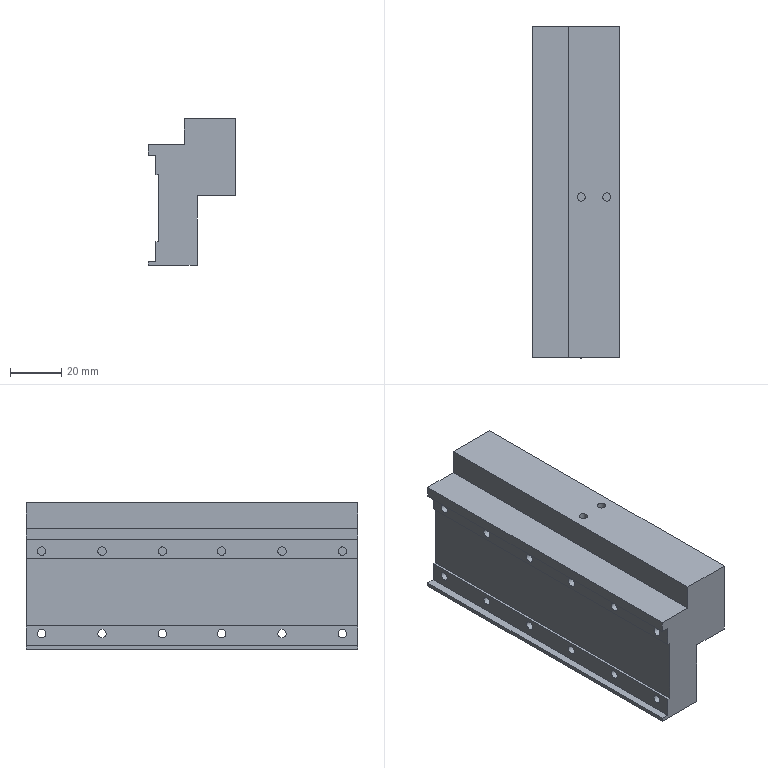Part | NX | 1 solid | 46 faces | box 34 x 129 x 57 mm | volume 157217 mm3 | plane 29 | cylinder 17 | commonest cylinder face diameters 3.3 x12 5 x3 3.2 x2
STEP:
#1=CARTESIAN_POINT('',(445.094,96.943,-207.9));
#2=VERTEX_POINT('',#1);
#3=CARTESIAN_POINT('',(446.694,96.943,-207.9));
#4=DIRECTION('',(0.,0.,-1.));
#5=DIRECTION('',(-1.,0.,0.));
#6=AXIS2_PLACEMENT_3D('',#3,#4,#5);
#7=CIRCLE('',#6,1.6);
#8=EDGE_CURVE('',#2,#2,#7,.T.);
#9=ORIENTED_EDGE('',*,*,#8,.F.);
#10=EDGE_LOOP('',(#9));
#11=FACE_BOUND('',#10,.T.);
#12=CARTESIAN_POINT('',(445.094,96.943,-215.9));
#13=VERTEX_POINT('',#12);
#14=CARTESIAN_POINT('',(446.694,96.943,-215.9));
#15=DIRECTION('',(0.,0.,-1.));
#16=DIRECTION('',(-1.,0.,0.));
#17=AXIS2_PLACEMENT_3D('',#14,#15,#16);
#18=CIRCLE('',#17,1.6);
#19=EDGE_CURVE('',#13,#13,#18,.T.);
#20=ORIENTED_EDGE('',*,*,#19,.T.);
#21=EDGE_LOOP('',(#20));
#22=FACE_BOUND('',#21,.T.);
#23=CARTESIAN_POINT('',(446.694,96.943,-207.9));
#24=DIRECTION('',(0.,0.,-1.));
#25=DIRECTION('',(-1.,0.,0.));
#26=AXIS2_PLACEMENT_3D('',#23,#24,#25);
#27=CYLINDRICAL_SURFACE('',#26,1.6);
#28=ADVANCED_FACE('',(#11,#22),#27,.F.);
#29=ORIENTED_EDGE('',*,*,#19,.F.);
#30=EDGE_LOOP('',(#29));
#31=FACE_BOUND('',#30,.T.);
#32=CARTESIAN_POINT('',(446.694,96.943,-215.9));
#33=DIRECTION('',(0.,0.,-1.));
#34=DIRECTION('',(1.,0.,0.));
#35=AXIS2_PLACEMENT_3D('',#32,#33,#34);
#36=PLANE('',#35);
#37=ADVANCED_FACE('',(#31),#36,.F.);
#38=CARTESIAN_POINT('',(455.094,96.943,-207.9));
#39=VERTEX_POINT('',#38);
#40=CARTESIAN_POINT('',(456.694,96.943,-207.9));
#41=DIRECTION('',(0.,0.,-1.));
#42=DIRECTION('',(-1.,0.,0.));
#43=AXIS2_PLACEMENT_3D('',#40,#41,#42);
#44=CIRCLE('',#43,1.6);
#45=EDGE_CURVE('',#39,#39,#44,.T.);
#46=ORIENTED_EDGE('',*,*,#45,.F.);
#47=EDGE_LOOP('',(#46));
#48=FACE_BOUND('',#47,.T.);
#49=CARTESIAN_POINT('',(455.094,96.943,-215.9));
#50=VERTEX_POINT('',#49);
#51=CARTESIAN_POINT('',(456.694,96.943,-215.9));
#52=DIRECTION('',(0.,0.,-1.));
#53=DIRECTION('',(-1.,0.,0.));
#54=AXIS2_PLACEMENT_3D('',#51,#52,#53);
#55=CIRCLE('',#54,1.6);
#56=EDGE_CURVE('',#50,#50,#55,.T.);
#57=ORIENTED_EDGE('',*,*,#56,.T.);
#58=EDGE_LOOP('',(#57));
#59=FACE_BOUND('',#58,.T.);
#60=CARTESIAN_POINT('',(456.694,96.943,-207.9));
#61=DIRECTION('',(0.,0.,-1.));
#62=DIRECTION('',(-1.,0.,0.));
#63=AXIS2_PLACEMENT_3D('',#60,#61,#62);
#64=CYLINDRICAL_SURFACE('',#63,1.6);
#65=ADVANCED_FACE('',(#48,#59),#64,.F.);
#66=ORIENTED_EDGE('',*,*,#56,.F.);
#67=EDGE_LOOP('',(#66));
#68=FACE_BOUND('',#67,.T.);
#69=CARTESIAN_POINT('',(446.694,96.943,-215.9));
#70=DIRECTION('',(0.,0.,-1.));
#71=DIRECTION('',(1.,0.,0.));
#72=AXIS2_PLACEMENT_3D('',#69,#70,#71);
#73=PLANE('',#72);
#74=ADVANCED_FACE('',(#68),#73,.F.);
#75=CARTESIAN_POINT('',(461.694,87.443,-228.377));
#76=VERTEX_POINT('',#75);
#77=CARTESIAN_POINT('',(461.694,87.443,-226.727));
#78=DIRECTION('',(1.,0.,0.));
#79=DIRECTION('',(0.,0.,-1.));
#80=AXIS2_PLACEMENT_3D('',#77,#78,#79);
#81=CIRCLE('',#80,1.65);
#82=EDGE_CURVE('',#76,#76,#81,.T.);
#83=ORIENTED_EDGE('',*,*,#82,.F.);
#84=EDGE_LOOP('',(#83));
#85=FACE_BOUND('',#84,.T.);
#86=CARTESIAN_POINT('',(461.694,133.943,-243.652));
#87=DIRECTION('',(1.,0.,0.));
#88=DIRECTION('',(0.,0.,1.));
#89=AXIS2_PLACEMENT_3D('',#86,#87,#88);
#90=PLANE('',#89);
#91=ADVANCED_FACE('',(#85),#90,.F.);
#92=CARTESIAN_POINT('',(461.694,63.943,-228.377));
#93=VERTEX_POINT('',#92);
#94=CARTESIAN_POINT('',(461.694,63.943,-226.727));
#95=DIRECTION('',(1.,0.,0.));
#96=DIRECTION('',(0.,0.,-1.));
#97=AXIS2_PLACEMENT_3D('',#94,#95,#96);
#98=CIRCLE('',#97,1.65);
#99=EDGE_CURVE('',#93,#93,#98,.T.);
#100=ORIENTED_EDGE('',*,*,#99,.F.);
#101=EDGE_LOOP('',(#100));
#102=FACE_BOUND('',#101,.T.);
#103=CARTESIAN_POINT('',(461.694,133.943,-243.652));
#104=DIRECTION('',(1.,0.,0.));
#105=DIRECTION('',(0.,0.,1.));
#106=AXIS2_PLACEMENT_3D('',#103,#104,#105);
#107=PLANE('',#106);
#108=ADVANCED_FACE('',(#102),#107,.F.);
#109=CARTESIAN_POINT('',(461.694,40.443,-228.377));
#110=VERTEX_POINT('',#109);
#111=CARTESIAN_POINT('',(461.694,40.443,-226.727));
#112=DIRECTION('',(1.,0.,0.));
#113=DIRECTION('',(0.,0.,-1.));
#114=AXIS2_PLACEMENT_3D('',#111,#112,#113);
#115=CIRCLE('',#114,1.65);
#116=EDGE_CURVE('',#110,#110,#115,.T.);
#117=ORIENTED_EDGE('',*,*,#116,.F.);
#118=EDGE_LOOP('',(#117));
#119=FACE_BOUND('',#118,.T.);
#120=CARTESIAN_POINT('',(461.694,133.943,-243.652));
#121=DIRECTION('',(1.,0.,0.));
#122=DIRECTION('',(0.,0.,1.));
#123=AXIS2_PLACEMENT_3D('',#120,#121,#122);
#124=PLANE('',#123);
#125=ADVANCED_FACE('',(#119),#124,.F.);
#126=CARTESIAN_POINT('',(461.694,157.443,-228.377));
#127=VERTEX_POINT('',#126);
#128=CARTESIAN_POINT('',(461.694,157.443,-226.727));
#129=DIRECTION('',(1.,0.,0.));
#130=DIRECTION('',(0.,0.,-1.));
#131=AXIS2_PLACEMENT_3D('',#128,#129,#130);
#132=CIRCLE('',#131,1.65);
#133=EDGE_CURVE('',#127,#127,#132,.T.);
#134=ORIENTED_EDGE('',*,*,#133,.F.);
#135=EDGE_LOOP('',(#134));
#136=FACE_BOUND('',#135,.T.);
#137=CARTESIAN_POINT('',(461.694,133.943,-243.652));
#138=DIRECTION('',(1.,0.,0.));
#139=DIRECTION('',(0.,0.,1.));
#140=AXIS2_PLACEMENT_3D('',#137,#138,#139);
#141=PLANE('',#140);
#142=ADVANCED_FACE('',(#136),#141,.F.);
#143=CARTESIAN_POINT('',(461.694,133.943,-228.377));
#144=VERTEX_POINT('',#143);
#145=CARTESIAN_POINT('',(461.694,133.943,-226.727));
#146=DIRECTION('',(1.,0.,0.));
#147=DIRECTION('',(0.,0.,-1.));
#148=AXIS2_PLACEMENT_3D('',#145,#146,#147);
#149=CIRCLE('',#148,1.65);
#150=EDGE_CURVE('',#144,#144,#149,.T.);
#151=ORIENTED_EDGE('',*,*,#150,.F.);
#152=EDGE_LOOP('',(#151));
#153=FACE_BOUND('',#152,.T.);
#154=CARTESIAN_POINT('',(461.694,133.943,-243.652));
#155=DIRECTION('',(1.,0.,0.));
#156=DIRECTION('',(0.,0.,1.));
#157=AXIS2_PLACEMENT_3D('',#154,#155,#156);
#158=PLANE('',#157);
#159=ADVANCED_FACE('',(#153),#158,.F.);
#160=CARTESIAN_POINT('',(461.694,110.443,-228.377));
#161=VERTEX_POINT('',#160);
#162=CARTESIAN_POINT('',(461.694,110.443,-226.727));
#163=DIRECTION('',(1.,0.,0.));
#164=DIRECTION('',(0.,0.,-1.));
#165=AXIS2_PLACEMENT_3D('',#162,#163,#164);
#166=CIRCLE('',#165,1.65);
#167=EDGE_CURVE('',#161,#161,#166,.T.);
#168=ORIENTED_EDGE('',*,*,#167,.F.);
#169=EDGE_LOOP('',(#168));
#170=FACE_BOUND('',#169,.T.);
#171=CARTESIAN_POINT('',(461.694,133.943,-243.652));
#172=DIRECTION('',(1.,0.,0.));
#173=DIRECTION('',(0.,0.,1.));
#174=AXIS2_PLACEMENT_3D('',#171,#172,#173);
#175=PLANE('',#174);
#176=ADVANCED_FACE('',(#170),#175,.F.);
#177=CARTESIAN_POINT('',(441.694,34.443,-207.9));
#178=VERTEX_POINT('',#177);
#179=CARTESIAN_POINT('',(461.694,34.443,-207.9));
#180=VERTEX_POINT('',#179);
#181=CARTESIAN_POINT('',(481.694,34.443,-207.9));
#182=DIRECTION('',(1.,0.,0.));
#183=VECTOR('',#182,1000.);
#184=LINE('',#181,#183);
#185=EDGE_CURVE('',#178,#180,#184,.T.);
#186=ORIENTED_EDGE('',*,*,#185,.T.);
#187=CARTESIAN_POINT('',(461.694,163.443,-207.9));
#188=VERTEX_POINT('',#187);
#189=CARTESIAN_POINT('',(461.694,681.443,-207.9));
#190=DIRECTION('',(0.,1.,0.));
#191=VECTOR('',#190,1000.);
#192=LINE('',#189,#191);
#193=EDGE_CURVE('',#180,#188,#192,.T.);
#194=ORIENTED_EDGE('',*,*,#193,.T.);
#195=CARTESIAN_POINT('',(441.694,163.443,-207.9));
#196=VERTEX_POINT('',#195);
#197=CARTESIAN_POINT('',(481.694,163.443,-207.9));
#198=DIRECTION('',(-1.,0.,0.));
#199=VECTOR('',#198,1000.);
#200=LINE('',#197,#199);
#201=EDGE_CURVE('',#188,#196,#200,.T.);
#202=ORIENTED_EDGE('',*,*,#201,.T.);
#203=CARTESIAN_POINT('',(441.694,681.443,-207.9));
#204=DIRECTION('',(0.,-1.,0.));
#205=VECTOR('',#204,1000.);
#206=LINE('',#203,#205);
#207=EDGE_CURVE('',#196,#178,#206,.T.);
#208=ORIENTED_EDGE('',*,*,#207,.T.);
#209=EDGE_LOOP('',(#186,#194,#202,#208));
#210=FACE_BOUND('',#209,.T.);
#211=ORIENTED_EDGE('',*,*,#45,.T.);
#212=EDGE_LOOP('',(#211));
#213=FACE_BOUND('',#212,.T.);
#214=ORIENTED_EDGE('',*,*,#8,.T.);
#215=EDGE_LOOP('',(#214));
#216=FACE_BOUND('',#215,.T.);
#217=CARTESIAN_POINT('',(481.694,681.443,-207.9));
#218=DIRECTION('',(0.,0.,-1.));
#219=DIRECTION('',(1.,0.,0.));
#220=AXIS2_PLACEMENT_3D('',#217,#218,#219);
#221=PLANE('',#220);
#222=ADVANCED_FACE('',(#210,#213,#216),#221,.F.);
#223=CARTESIAN_POINT('',(461.694,34.443,-237.9));
#224=VERTEX_POINT('',#223);
#225=CARTESIAN_POINT('',(461.694,163.443,-237.9));
#226=VERTEX_POINT('',#225);
#227=CARTESIAN_POINT('',(461.694,133.943,-237.9));
#228=DIRECTION('',(0.,1.,0.));
#229=VECTOR('',#228,1000.);
#230=LINE('',#227,#229);
#231=EDGE_CURVE('',#224,#226,#230,.T.);
#232=ORIENTED_EDGE('',*,*,#231,.T.);
#233=CARTESIAN_POINT('',(461.694,163.443,-213.827));
#234=DIRECTION('',(0.,0.,-1.));
#235=VECTOR('',#234,1000.);
#236=LINE('',#233,#235);
#237=EDGE_CURVE('',#188,#226,#236,.T.);
#238=ORIENTED_EDGE('',*,*,#237,.F.);
#239=ORIENTED_EDGE('',*,*,#193,.F.);
#240=CARTESIAN_POINT('',(461.694,34.443,-452.827));
#241=DIRECTION('',(0.,0.,1.));
#242=VECTOR('',#241,1000.);
#243=LINE('',#240,#242);
#244=EDGE_CURVE('',#224,#180,#243,.T.);
#245=ORIENTED_EDGE('',*,*,#244,.F.);
#246=EDGE_LOOP('',(#232,#238,#239,#245));
#247=FACE_BOUND('',#246,.T.);
#248=CARTESIAN_POINT('',(461.694,143.443,-225.4));
#249=VERTEX_POINT('',#248);
#250=CARTESIAN_POINT('',(461.694,143.443,-222.9));
#251=DIRECTION('',(-1.,0.,0.));
#252=DIRECTION('',(0.,0.,-1.));
#253=AXIS2_PLACEMENT_3D('',#250,#251,#252);
#254=CIRCLE('',#253,2.5);
#255=EDGE_CURVE('',#249,#249,#254,.T.);
#256=ORIENTED_EDGE('',*,*,#255,.T.);
#257=EDGE_LOOP('',(#256));
#258=FACE_BOUND('',#257,.T.);
#259=CARTESIAN_POINT('',(461.694,98.943,-225.4));
#260=VERTEX_POINT('',#259);
#261=CARTESIAN_POINT('',(461.694,98.943,-222.9));
#262=DIRECTION('',(-1.,0.,0.));
#263=DIRECTION('',(0.,0.,-1.));
#264=AXIS2_PLACEMENT_3D('',#261,#262,#263);
#265=CIRCLE('',#264,2.5);
#266=EDGE_CURVE('',#260,#260,#265,.T.);
#267=ORIENTED_EDGE('',*,*,#266,.T.);
#268=EDGE_LOOP('',(#267));
#269=FACE_BOUND('',#268,.T.);
#270=CARTESIAN_POINT('',(461.694,54.443,-225.4));
#271=VERTEX_POINT('',#270);
#272=CARTESIAN_POINT('',(461.694,54.443,-222.9));
#273=DIRECTION('',(-1.,0.,0.));
#274=DIRECTION('',(0.,0.,-1.));
#275=AXIS2_PLACEMENT_3D('',#272,#273,#274);
#276=CIRCLE('',#275,2.5);
#277=EDGE_CURVE('',#271,#271,#276,.T.);
#278=ORIENTED_EDGE('',*,*,#277,.T.);
#279=EDGE_LOOP('',(#278));
#280=FACE_BOUND('',#279,.T.);
#281=CARTESIAN_POINT('',(461.694,133.943,-243.652));
#282=DIRECTION('',(1.,0.,0.));
#283=DIRECTION('',(0.,0.,1.));
#284=AXIS2_PLACEMENT_3D('',#281,#282,#283);
#285=PLANE('',#284);
#286=ADVANCED_FACE('',(#247,#258,#269,#280),#285,.T.);
#287=CARTESIAN_POINT('',(446.694,163.443,-237.9));
#288=VERTEX_POINT('',#287);
#289=CARTESIAN_POINT('',(446.694,34.443,-237.9));
#290=VERTEX_POINT('',#289);
#291=CARTESIAN_POINT('',(446.694,731.443,-237.9));
#292=DIRECTION('',(0.,-1.,0.));
#293=VECTOR('',#292,1000.);
#294=LINE('',#291,#293);
#295=EDGE_CURVE('',#288,#290,#294,.T.);
#296=ORIENTED_EDGE('',*,*,#295,.F.);
#297=CARTESIAN_POINT('',(488.694,163.443,-237.9));
#298=DIRECTION('',(-1.,0.,0.));
#299=VECTOR('',#298,1000.);
#300=LINE('',#297,#299);
#301=EDGE_CURVE('',#226,#288,#300,.T.);
#302=ORIENTED_EDGE('',*,*,#301,.F.);
#303=ORIENTED_EDGE('',*,*,#231,.F.);
#304=CARTESIAN_POINT('',(459.484,34.443,-237.9));
#305=DIRECTION('',(-1.,0.,0.));
#306=VECTOR('',#305,1000.);
#307=LINE('',#304,#306);
#308=EDGE_CURVE('',#224,#290,#307,.T.);
#309=ORIENTED_EDGE('',*,*,#308,.T.);
#310=EDGE_LOOP('',(#296,#302,#303,#309));
#311=FACE_BOUND('',#310,.T.);
#312=CARTESIAN_POINT('',(488.694,731.443,-237.9));
#313=DIRECTION('',(0.,0.,-1.));
#314=DIRECTION('',(1.,0.,0.));
#315=AXIS2_PLACEMENT_3D('',#312,#313,#314);
#316=PLANE('',#315);
#317=ADVANCED_FACE('',(#311),#316,.T.);
#318=CARTESIAN_POINT('',(451.694,143.443,-220.4));
#319=VERTEX_POINT('',#318);
#320=CARTESIAN_POINT('',(451.694,143.443,-222.9));
#321=DIRECTION('',(-1.,0.,0.));
#322=DIRECTION('',(0.,0.,1.));
#323=AXIS2_PLACEMENT_3D('',#320,#321,#322);
#324=CIRCLE('',#323,2.5);
#325=EDGE_CURVE('',#319,#319,#324,.T.);
#326=ORIENTED_EDGE('',*,*,#325,.F.);
#327=EDGE_LOOP('',(#326));
#328=FACE_BOUND('',#327,.T.);
#329=CARTESIAN_POINT('',(451.694,143.443,-222.9));
#330=DIRECTION('',(-1.,0.,0.));
#331=DIRECTION('',(0.,0.,-1.));
#332=AXIS2_PLACEMENT_3D('',#329,#330,#331);
#333=PLANE('',#332);
#334=ADVANCED_FACE('',(#328),#333,.F.);
#335=ORIENTED_EDGE('',*,*,#255,.F.);
#336=EDGE_LOOP('',(#335));
#337=FACE_BOUND('',#336,.T.);
#338=ORIENTED_EDGE('',*,*,#325,.T.);
#339=EDGE_LOOP('',(#338));
#340=FACE_BOUND('',#339,.T.);
#341=CARTESIAN_POINT('',(481.694,143.443,-222.9));
#342=DIRECTION('',(-1.,0.,0.));
#343=DIRECTION('',(0.,0.,-1.));
#344=AXIS2_PLACEMENT_3D('',#341,#342,#343);
#345=CYLINDRICAL_SURFACE('',#344,2.5);
#346=ADVANCED_FACE('',(#337,#340),#345,.F.);
#347=CARTESIAN_POINT('',(451.694,98.943,-220.4));
#348=VERTEX_POINT('',#347);
#349=CARTESIAN_POINT('',(451.694,98.943,-222.9));
#350=DIRECTION('',(-1.,0.,0.));
#351=DIRECTION('',(0.,0.,1.));
#352=AXIS2_PLACEMENT_3D('',#349,#350,#351);
#353=CIRCLE('',#352,2.5);
#354=EDGE_CURVE('',#348,#348,#353,.T.);
#355=ORIENTED_EDGE('',*,*,#354,.F.);
#356=EDGE_LOOP('',(#355));
#357=FACE_BOUND('',#356,.T.);
#358=CARTESIAN_POINT('',(451.694,143.443,-222.9));
#359=DIRECTION('',(-1.,0.,0.));
#360=DIRECTION('',(0.,0.,-1.));
#361=AXIS2_PLACEMENT_3D('',#358,#359,#360);
#362=PLANE('',#361);
#363=ADVANCED_FACE('',(#357),#362,.F.);
#364=ORIENTED_EDGE('',*,*,#266,.F.);
#365=EDGE_LOOP('',(#364));
#366=FACE_BOUND('',#365,.T.);
#367=ORIENTED_EDGE('',*,*,#354,.T.);
#368=EDGE_LOOP('',(#367));
#369=FACE_BOUND('',#368,.T.);
#370=CARTESIAN_POINT('',(481.694,98.943,-222.9));
#371=DIRECTION('',(-1.,0.,0.));
#372=DIRECTION('',(0.,0.,-1.));
#373=AXIS2_PLACEMENT_3D('',#370,#371,#372);
#374=CYLINDRICAL_SURFACE('',#373,2.5);
#375=ADVANCED_FACE('',(#366,#369),#374,.F.);
#376=CARTESIAN_POINT('',(451.694,54.443,-220.4));
#377=VERTEX_POINT('',#376);
#378=CARTESIAN_POINT('',(451.694,54.443,-222.9));
#379=DIRECTION('',(-1.,0.,0.));
#380=DIRECTION('',(0.,0.,1.));
#381=AXIS2_PLACEMENT_3D('',#378,#379,#380);
#382=CIRCLE('',#381,2.5);
#383=EDGE_CURVE('',#377,#377,#382,.T.);
#384=ORIENTED_EDGE('',*,*,#383,.F.);
#385=EDGE_LOOP('',(#384));
#386=FACE_BOUND('',#385,.T.);
#387=CARTESIAN_POINT('',(451.694,143.443,-222.9));
#388=DIRECTION('',(-1.,0.,0.));
#389=DIRECTION('',(0.,0.,-1.));
#390=AXIS2_PLACEMENT_3D('',#387,#388,#389);
#391=PLANE('',#390);
#392=ADVANCED_FACE('',(#386),#391,.F.);
#393=ORIENTED_EDGE('',*,*,#277,.F.);
#394=EDGE_LOOP('',(#393));
#395=FACE_BOUND('',#394,.T.);
#396=ORIENTED_EDGE('',*,*,#383,.T.);
#397=EDGE_LOOP('',(#396));
#398=FACE_BOUND('',#397,.T.);
#399=CARTESIAN_POINT('',(481.694,54.443,-222.9));
#400=DIRECTION('',(-1.,0.,0.));
#401=DIRECTION('',(0.,0.,-1.));
#402=AXIS2_PLACEMENT_3D('',#399,#400,#401);
#403=CYLINDRICAL_SURFACE('',#402,2.5);
#404=ADVANCED_FACE('',(#395,#398),#403,.F.);
#405=CARTESIAN_POINT('',(441.694,34.443,-217.9));
#406=VERTEX_POINT('',#405);
#407=CARTESIAN_POINT('',(441.694,163.443,-217.9));
#408=VERTEX_POINT('',#407);
#409=CARTESIAN_POINT('',(441.694,133.943,-217.9));
#410=DIRECTION('',(0.,1.,0.));
#411=VECTOR('',#410,1000.);
#412=LINE('',#409,#411);
#413=EDGE_CURVE('',#406,#408,#412,.T.);
#414=ORIENTED_EDGE('',*,*,#413,.F.);
#415=CARTESIAN_POINT('',(441.694,34.443,-452.827));
#416=DIRECTION('',(0.,0.,-1.));
#417=VECTOR('',#416,1000.);
#418=LINE('',#415,#417);
#419=EDGE_CURVE('',#178,#406,#418,.T.);
#420=ORIENTED_EDGE('',*,*,#419,.F.);
#421=ORIENTED_EDGE('',*,*,#207,.F.);
#422=CARTESIAN_POINT('',(441.694,163.443,-213.827));
#423=DIRECTION('',(0.,0.,1.));
#424=VECTOR('',#423,1000.);
#425=LINE('',#422,#424);
#426=EDGE_CURVE('',#408,#196,#425,.T.);
#427=ORIENTED_EDGE('',*,*,#426,.F.);
#428=EDGE_LOOP('',(#414,#420,#421,#427));
#429=FACE_BOUND('',#428,.T.);
#430=CARTESIAN_POINT('',(441.694,133.943,-243.652));
#431=DIRECTION('',(1.,0.,0.));
#432=DIRECTION('',(0.,0.,1.));
#433=AXIS2_PLACEMENT_3D('',#430,#431,#432);
#434=PLANE('',#433);
#435=ADVANCED_FACE('',(#429),#434,.F.);
#436=CARTESIAN_POINT('',(446.694,163.443,-264.9));
#437=VERTEX_POINT('',#436);
#438=CARTESIAN_POINT('',(446.694,163.443,-251.4));
#439=DIRECTION('',(0.,0.,-1.));
#440=VECTOR('',#439,1000.);
#441=LINE('',#438,#440);
#442=EDGE_CURVE('',#288,#437,#441,.T.);
#443=ORIENTED_EDGE('',*,*,#442,.T.);
#444=CARTESIAN_POINT('',(427.694,163.443,-264.9));
#445=VERTEX_POINT('',#444);
#446=CARTESIAN_POINT('',(454.484,163.443,-264.9));
#447=DIRECTION('',(1.,0.,0.));
#448=VECTOR('',#447,1000.);
#449=LINE('',#446,#448);
#450=EDGE_CURVE('',#445,#437,#449,.T.);
#451=ORIENTED_EDGE('',*,*,#450,.F.);
#452=CARTESIAN_POINT('',(427.694,163.443,-263.427));
#453=VERTEX_POINT('',#452);
#454=CARTESIAN_POINT('',(427.694,163.443,-213.827));
#455=DIRECTION('',(0.,0.,1.));
#456=VECTOR('',#455,1000.);
#457=LINE('',#454,#456);
#458=EDGE_CURVE('',#445,#453,#457,.T.);
#459=ORIENTED_EDGE('',*,*,#458,.T.);
#460=CARTESIAN_POINT('',(430.694,163.443,-263.427));
#461=VERTEX_POINT('',#460);
#462=CARTESIAN_POINT('',(427.599,163.443,-263.427));
#463=DIRECTION('',(-1.,0.,0.));
#464=VECTOR('',#463,1000.);
#465=LINE('',#462,#464);
#466=EDGE_CURVE('',#461,#453,#465,.T.);
#467=ORIENTED_EDGE('',*,*,#466,.F.);
#468=CARTESIAN_POINT('',(430.694,163.443,-255.827));
#469=VERTEX_POINT('',#468);
#470=CARTESIAN_POINT('',(430.694,163.443,-213.827));
#471=DIRECTION('',(0.,0.,1.));
#472=VECTOR('',#471,1000.);
#473=LINE('',#470,#472);
#474=EDGE_CURVE('',#461,#469,#473,.T.);
#475=ORIENTED_EDGE('',*,*,#474,.T.);
#476=CARTESIAN_POINT('',(431.694,163.443,-255.827));
#477=VERTEX_POINT('',#476);
#478=CARTESIAN_POINT('',(439.484,163.443,-255.827));
#479=DIRECTION('',(1.,0.,0.));
#480=VECTOR('',#479,1000.);
#481=LINE('',#478,#480);
#482=EDGE_CURVE('',#469,#477,#481,.T.);
#483=ORIENTED_EDGE('',*,*,#482,.T.);
#484=CARTESIAN_POINT('',(431.694,163.443,-229.727));
#485=VERTEX_POINT('',#484);
#486=CARTESIAN_POINT('',(431.694,163.443,-213.827));
#487=DIRECTION('',(0.,0.,-1.));
#488=VECTOR('',#487,1000.);
#489=LINE('',#486,#488);
#490=EDGE_CURVE('',#485,#477,#489,.T.);
#491=ORIENTED_EDGE('',*,*,#490,.F.);
#492=CARTESIAN_POINT('',(430.694,163.443,-229.727));
#493=VERTEX_POINT('',#492);
#494=CARTESIAN_POINT('',(439.484,163.443,-229.727));
#495=DIRECTION('',(1.,0.,0.));
#496=VECTOR('',#495,1000.);
#497=LINE('',#494,#496);
#498=EDGE_CURVE('',#493,#485,#497,.T.);
#499=ORIENTED_EDGE('',*,*,#498,.F.);
#500=CARTESIAN_POINT('',(430.694,163.443,-222.127));
#501=VERTEX_POINT('',#500);
#502=CARTESIAN_POINT('',(430.694,163.443,-242.827));
#503=DIRECTION('',(0.,0.,-1.));
#504=VECTOR('',#503,1000.);
#505=LINE('',#502,#504);
#506=EDGE_CURVE('',#501,#493,#505,.T.);
#507=ORIENTED_EDGE('',*,*,#506,.F.);
#508=CARTESIAN_POINT('',(427.694,163.443,-222.127));
#509=VERTEX_POINT('',#508);
#510=CARTESIAN_POINT('',(427.599,163.443,-222.127));
#511=DIRECTION('',(-1.,0.,0.));
#512=VECTOR('',#511,1000.);
#513=LINE('',#510,#512);
#514=EDGE_CURVE('',#501,#509,#513,.T.);
#515=ORIENTED_EDGE('',*,*,#514,.T.);
#516=CARTESIAN_POINT('',(427.694,163.443,-217.9));
#517=VERTEX_POINT('',#516);
#518=CARTESIAN_POINT('',(427.694,163.443,-271.727));
#519=DIRECTION('',(0.,0.,-1.));
#520=VECTOR('',#519,1000.);
#521=LINE('',#518,#520);
#522=EDGE_CURVE('',#517,#509,#521,.T.);
#523=ORIENTED_EDGE('',*,*,#522,.F.);
#524=CARTESIAN_POINT('',(481.694,163.443,-217.9));
#525=DIRECTION('',(-1.,0.,0.));
#526=VECTOR('',#525,1000.);
#527=LINE('',#524,#526);
#528=EDGE_CURVE('',#408,#517,#527,.T.);
#529=ORIENTED_EDGE('',*,*,#528,.F.);
#530=ORIENTED_EDGE('',*,*,#426,.T.);
#531=ORIENTED_EDGE('',*,*,#201,.F.);
#532=ORIENTED_EDGE('',*,*,#237,.T.);
#533=ORIENTED_EDGE('',*,*,#301,.T.);
#534=EDGE_LOOP('',(#443,#451,#459,#467,#475,#483,#491,#499,#507,#515,#523,#529,#530,#531,#532,#533));
#535=FACE_BOUND('',#534,.T.);
#536=CARTESIAN_POINT('',(454.484,163.443,-213.827));
#537=DIRECTION('',(0.,-1.,0.));
#538=DIRECTION('',(1.,0.,0.));
#539=AXIS2_PLACEMENT_3D('',#536,#537,#538);
#540=PLANE('',#539);
#541=ADVANCED_FACE('',(#535),#540,.F.);
#542=CARTESIAN_POINT('',(427.694,34.443,-217.9));
#543=VERTEX_POINT('',#542);
#544=CARTESIAN_POINT('',(481.694,34.443,-217.9));
#545=DIRECTION('',(1.,0.,0.));
#546=VECTOR('',#545,1000.);
#547=LINE('',#544,#546);
#548=EDGE_CURVE('',#543,#406,#547,.T.);
#549=ORIENTED_EDGE('',*,*,#548,.F.);
#550=CARTESIAN_POINT('',(427.694,34.443,-222.127));
#551=VERTEX_POINT('',#550);
#552=CARTESIAN_POINT('',(427.694,34.443,-32.727));
#553=DIRECTION('',(0.,0.,1.));
#554=VECTOR('',#553,1000.);
#555=LINE('',#552,#554);
#556=EDGE_CURVE('',#551,#543,#555,.T.);
#557=ORIENTED_EDGE('',*,*,#556,.F.);
#558=CARTESIAN_POINT('',(430.694,34.443,-222.127));
#559=VERTEX_POINT('',#558);
#560=CARTESIAN_POINT('',(444.484,34.443,-222.127));
#561=DIRECTION('',(-1.,0.,0.));
#562=VECTOR('',#561,1000.);
#563=LINE('',#560,#562);
#564=EDGE_CURVE('',#559,#551,#563,.T.);
#565=ORIENTED_EDGE('',*,*,#564,.F.);
#566=CARTESIAN_POINT('',(430.694,34.443,-229.727));
#567=VERTEX_POINT('',#566);
#568=CARTESIAN_POINT('',(430.694,34.443,-242.827));
#569=DIRECTION('',(0.,0.,1.));
#570=VECTOR('',#569,1000.);
#571=LINE('',#568,#570);
#572=EDGE_CURVE('',#567,#559,#571,.T.);
#573=ORIENTED_EDGE('',*,*,#572,.F.);
#574=CARTESIAN_POINT('',(431.694,34.443,-229.727));
#575=VERTEX_POINT('',#574);
#576=CARTESIAN_POINT('',(444.484,34.443,-229.727));
#577=DIRECTION('',(-1.,0.,0.));
#578=VECTOR('',#577,1000.);
#579=LINE('',#576,#578);
#580=EDGE_CURVE('',#575,#567,#579,.T.);
#581=ORIENTED_EDGE('',*,*,#580,.F.);
#582=CARTESIAN_POINT('',(431.694,34.443,-255.827));
#583=VERTEX_POINT('',#582);
#584=CARTESIAN_POINT('',(431.694,34.443,-452.827));
#585=DIRECTION('',(0.,0.,1.));
#586=VECTOR('',#585,1000.);
#587=LINE('',#584,#586);
#588=EDGE_CURVE('',#583,#575,#587,.T.);
#589=ORIENTED_EDGE('',*,*,#588,.F.);
#590=CARTESIAN_POINT('',(430.694,34.443,-255.827));
#591=VERTEX_POINT('',#590);
#592=CARTESIAN_POINT('',(444.484,34.443,-255.827));
#593=DIRECTION('',(-1.,0.,0.));
#594=VECTOR('',#593,1000.);
#595=LINE('',#592,#594);
#596=EDGE_CURVE('',#583,#591,#595,.T.);
#597=ORIENTED_EDGE('',*,*,#596,.T.);
#598=CARTESIAN_POINT('',(430.694,34.443,-263.427));
#599=VERTEX_POINT('',#598);
#600=CARTESIAN_POINT('',(430.694,34.443,-452.827));
#601=DIRECTION('',(0.,0.,-1.));
#602=VECTOR('',#601,1000.);
#603=LINE('',#600,#602);
#604=EDGE_CURVE('',#591,#599,#603,.T.);
#605=ORIENTED_EDGE('',*,*,#604,.T.);
#606=CARTESIAN_POINT('',(427.694,34.443,-263.427));
#607=VERTEX_POINT('',#606);
#608=CARTESIAN_POINT('',(444.484,34.443,-263.427));
#609=DIRECTION('',(-1.,0.,0.));
#610=VECTOR('',#609,1000.);
#611=LINE('',#608,#610);
#612=EDGE_CURVE('',#599,#607,#611,.T.);
#613=ORIENTED_EDGE('',*,*,#612,.T.);
#614=CARTESIAN_POINT('',(427.694,34.443,-264.9));
#615=VERTEX_POINT('',#614);
#616=CARTESIAN_POINT('',(427.694,34.443,-452.827));
#617=DIRECTION('',(0.,0.,-1.));
#618=VECTOR('',#617,1000.);
#619=LINE('',#616,#618);
#620=EDGE_CURVE('',#607,#615,#619,.T.);
#621=ORIENTED_EDGE('',*,*,#620,.T.);
#622=CARTESIAN_POINT('',(446.694,34.443,-264.9));
#623=VERTEX_POINT('',#622);
#624=CARTESIAN_POINT('',(459.484,34.443,-264.9));
#625=DIRECTION('',(1.,0.,0.));
#626=VECTOR('',#625,1000.);
#627=LINE('',#624,#626);
#628=EDGE_CURVE('',#615,#623,#627,.T.);
#629=ORIENTED_EDGE('',*,*,#628,.T.);
#630=CARTESIAN_POINT('',(446.694,34.443,-251.4));
#631=DIRECTION('',(0.,0.,1.));
#632=VECTOR('',#631,1000.);
#633=LINE('',#630,#632);
#634=EDGE_CURVE('',#623,#290,#633,.T.);
#635=ORIENTED_EDGE('',*,*,#634,.T.);
#636=ORIENTED_EDGE('',*,*,#308,.F.);
#637=ORIENTED_EDGE('',*,*,#244,.T.);
#638=ORIENTED_EDGE('',*,*,#185,.F.);
#639=ORIENTED_EDGE('',*,*,#419,.T.);
#640=EDGE_LOOP('',(#549,#557,#565,#573,#581,#589,#597,#605,#613,#621,#629,#635,#636,#637,#638,#639));
#641=FACE_BOUND('',#640,.T.);
#642=CARTESIAN_POINT('',(459.484,34.443,-452.827));
#643=DIRECTION('',(0.,1.,0.));
#644=DIRECTION('',(1.,0.,0.));
#645=AXIS2_PLACEMENT_3D('',#642,#643,#644);
#646=PLANE('',#645);
#647=ADVANCED_FACE('',(#641),#646,.F.);
#648=ORIENTED_EDGE('',*,*,#413,.T.);
#649=ORIENTED_EDGE('',*,*,#528,.T.);
#650=CARTESIAN_POINT('',(427.694,100.193,-217.9));
#651=DIRECTION('',(0.,1.,0.));
#652=VECTOR('',#651,1000.);
#653=LINE('',#650,#652);
#654=EDGE_CURVE('',#543,#517,#653,.T.);
#655=ORIENTED_EDGE('',*,*,#654,.F.);
#656=ORIENTED_EDGE('',*,*,#548,.T.);
#657=EDGE_LOOP('',(#648,#649,#655,#656));
#658=FACE_BOUND('',#657,.T.);
#659=CARTESIAN_POINT('',(481.694,681.443,-217.9));
#660=DIRECTION('',(0.,0.,-1.));
#661=DIRECTION('',(1.,0.,0.));
#662=AXIS2_PLACEMENT_3D('',#659,#660,#661);
#663=PLANE('',#662);
#664=ADVANCED_FACE('',(#658),#663,.F.);
#665=ORIENTED_EDGE('',*,*,#654,.T.);
#666=ORIENTED_EDGE('',*,*,#522,.T.);
#667=CARTESIAN_POINT('',(427.694,100.193,-222.127));
#668=DIRECTION('',(0.,1.,0.));
#669=VECTOR('',#668,1000.);
#670=LINE('',#667,#669);
#671=EDGE_CURVE('',#551,#509,#670,.T.);
#672=ORIENTED_EDGE('',*,*,#671,.F.);
#673=ORIENTED_EDGE('',*,*,#556,.T.);
#674=EDGE_LOOP('',(#665,#666,#672,#673));
#675=FACE_BOUND('',#674,.T.);
#676=CARTESIAN_POINT('',(427.694,100.193,-242.727));
#677=DIRECTION('',(1.,0.,0.));
#678=DIRECTION('',(0.,-1.,0.));
#679=AXIS2_PLACEMENT_3D('',#676,#677,#678);
#680=PLANE('',#679);
#681=ADVANCED_FACE('',(#675),#680,.F.);
#682=CARTESIAN_POINT('',(446.694,98.943,-264.9));
#683=DIRECTION('',(0.,1.,0.));
#684=VECTOR('',#683,1000.);
#685=LINE('',#682,#684);
#686=EDGE_CURVE('',#623,#437,#685,.T.);
#687=ORIENTED_EDGE('',*,*,#686,.F.);
#688=ORIENTED_EDGE('',*,*,#628,.F.);
#689=CARTESIAN_POINT('',(427.694,98.943,-264.9));
#690=DIRECTION('',(0.,1.,0.));
#691=VECTOR('',#690,1000.);
#692=LINE('',#689,#691);
#693=EDGE_CURVE('',#615,#445,#692,.T.);
#694=ORIENTED_EDGE('',*,*,#693,.T.);
#695=ORIENTED_EDGE('',*,*,#450,.T.);
#696=EDGE_LOOP('',(#687,#688,#694,#695));
#697=FACE_BOUND('',#696,.T.);
#698=CARTESIAN_POINT('',(471.694,98.943,-264.9));
#699=DIRECTION('',(0.,0.,-1.));
#700=DIRECTION('',(1.,0.,0.));
#701=AXIS2_PLACEMENT_3D('',#698,#699,#700);
#702=PLANE('',#701);
#703=ADVANCED_FACE('',(#697),#702,.T.);
#704=ORIENTED_EDGE('',*,*,#693,.F.);
#705=ORIENTED_EDGE('',*,*,#620,.F.);
#706=CARTESIAN_POINT('',(427.694,100.193,-263.427));
#707=DIRECTION('',(0.,1.,0.));
#708=VECTOR('',#707,1000.);
#709=LINE('',#706,#708);
#710=EDGE_CURVE('',#607,#453,#709,.T.);
#711=ORIENTED_EDGE('',*,*,#710,.T.);
#712=ORIENTED_EDGE('',*,*,#458,.F.);
#713=EDGE_LOOP('',(#704,#705,#711,#712));
#714=FACE_BOUND('',#713,.T.);
#715=CARTESIAN_POINT('',(427.694,100.193,-242.727));
#716=DIRECTION('',(1.,0.,0.));
#717=DIRECTION('',(0.,-1.,0.));
#718=AXIS2_PLACEMENT_3D('',#715,#716,#717);
#719=PLANE('',#718);
#720=ADVANCED_FACE('',(#714),#719,.F.);
#721=ORIENTED_EDGE('',*,*,#710,.F.);
#722=ORIENTED_EDGE('',*,*,#612,.F.);
#723=CARTESIAN_POINT('',(430.694,133.943,-263.427));
#724=DIRECTION('',(0.,-1.,0.));
#725=VECTOR('',#724,1000.);
#726=LINE('',#723,#725);
#727=EDGE_CURVE('',#461,#599,#726,.T.);
#728=ORIENTED_EDGE('',*,*,#727,.F.);
#729=ORIENTED_EDGE('',*,*,#466,.T.);
#730=EDGE_LOOP('',(#721,#722,#728,#729));
#731=FACE_BOUND('',#730,.T.);
#732=CARTESIAN_POINT('',(427.599,133.943,-263.427));
#733=DIRECTION('',(0.,0.,-1.));
#734=DIRECTION('',(0.,-1.,0.));
#735=AXIS2_PLACEMENT_3D('',#732,#733,#734);
#736=PLANE('',#735);
#737=ADVANCED_FACE('',(#731),#736,.F.);
#738=CARTESIAN_POINT('',(430.694,87.443,-260.477));
#739=VERTEX_POINT('',#738);
#740=CARTESIAN_POINT('',(430.694,87.443,-258.827));
#741=DIRECTION('',(1.,0.,0.));
#742=DIRECTION('',(0.,0.,-1.));
#743=AXIS2_PLACEMENT_3D('',#740,#741,#742);
#744=CIRCLE('',#743,1.65);
#745=EDGE_CURVE('',#739,#739,#744,.T.);
#746=ORIENTED_EDGE('',*,*,#745,.T.);
#747=EDGE_LOOP('',(#746));
#748=FACE_BOUND('',#747,.T.);
#749=CARTESIAN_POINT('',(430.694,63.943,-260.477));
#750=VERTEX_POINT('',#749);
#751=CARTESIAN_POINT('',(430.694,63.943,-258.827));
#752=DIRECTION('',(1.,0.,0.));
#753=DIRECTION('',(0.,0.,-1.));
#754=AXIS2_PLACEMENT_3D('',#751,#752,#753);
#755=CIRCLE('',#754,1.65);
#756=EDGE_CURVE('',#750,#750,#755,.T.);
#757=ORIENTED_EDGE('',*,*,#756,.T.);
#758=EDGE_LOOP('',(#757));
#759=FACE_BOUND('',#758,.T.);
#760=CARTESIAN_POINT('',(430.694,40.443,-260.477));
#761=VERTEX_POINT('',#760);
#762=CARTESIAN_POINT('',(430.694,40.443,-258.827));
#763=DIRECTION('',(1.,0.,0.));
#764=DIRECTION('',(0.,0.,-1.));
#765=AXIS2_PLACEMENT_3D('',#762,#763,#764);
#766=CIRCLE('',#765,1.65);
#767=EDGE_CURVE('',#761,#761,#766,.T.);
#768=ORIENTED_EDGE('',*,*,#767,.T.);
#769=EDGE_LOOP('',(#768));
#770=FACE_BOUND('',#769,.T.);
#771=CARTESIAN_POINT('',(430.694,157.443,-260.477));
#772=VERTEX_POINT('',#771);
#773=CARTESIAN_POINT('',(430.694,157.443,-258.827));
#774=DIRECTION('',(1.,0.,0.));
#775=DIRECTION('',(0.,0.,-1.));
#776=AXIS2_PLACEMENT_3D('',#773,#774,#775);
#777=CIRCLE('',#776,1.65);
#778=EDGE_CURVE('',#772,#772,#777,.T.);
#779=ORIENTED_EDGE('',*,*,#778,.T.);
#780=EDGE_LOOP('',(#779));
#781=FACE_BOUND('',#780,.T.);
#782=CARTESIAN_POINT('',(430.694,133.943,-260.477));
#783=VERTEX_POINT('',#782);
#784=CARTESIAN_POINT('',(430.694,133.943,-258.827));
#785=DIRECTION('',(1.,0.,0.));
#786=DIRECTION('',(0.,0.,-1.));
#787=AXIS2_PLACEMENT_3D('',#784,#785,#786);
#788=CIRCLE('',#787,1.65);
#789=EDGE_CURVE('',#783,#783,#788,.T.);
#790=ORIENTED_EDGE('',*,*,#789,.T.);
#791=EDGE_LOOP('',(#790));
#792=FACE_BOUND('',#791,.T.);
#793=CARTESIAN_POINT('',(430.694,110.443,-260.477));
#794=VERTEX_POINT('',#793);
#795=CARTESIAN_POINT('',(430.694,110.443,-258.827));
#796=DIRECTION('',(1.,0.,0.));
#797=DIRECTION('',(0.,0.,-1.));
#798=AXIS2_PLACEMENT_3D('',#795,#796,#797);
#799=CIRCLE('',#798,1.65);
#800=EDGE_CURVE('',#794,#794,#799,.T.);
#801=ORIENTED_EDGE('',*,*,#800,.T.);
#802=EDGE_LOOP('',(#801));
#803=FACE_BOUND('',#802,.T.);
#804=ORIENTED_EDGE('',*,*,#727,.T.);
#805=ORIENTED_EDGE('',*,*,#604,.F.);
#806=CARTESIAN_POINT('',(430.694,353.693,-255.827));
#807=DIRECTION('',(0.,-1.,0.));
#808=VECTOR('',#807,1000.);
#809=LINE('',#806,#808);
#810=EDGE_CURVE('',#469,#591,#809,.T.);
#811=ORIENTED_EDGE('',*,*,#810,.F.);
#812=ORIENTED_EDGE('',*,*,#474,.F.);
#813=EDGE_LOOP('',(#804,#805,#811,#812));
#814=FACE_BOUND('',#813,.T.);
#815=CARTESIAN_POINT('',(430.694,100.193,-242.827));
#816=DIRECTION('',(1.,0.,0.));
#817=DIRECTION('',(0.,-1.,0.));
#818=AXIS2_PLACEMENT_3D('',#815,#816,#817);
#819=PLANE('',#818);
#820=ADVANCED_FACE('',(#748,#759,#770,#781,#792,#803,#814),#819,.F.);
#821=ORIENTED_EDGE('',*,*,#482,.F.);
#822=ORIENTED_EDGE('',*,*,#810,.T.);
#823=ORIENTED_EDGE('',*,*,#596,.F.);
#824=CARTESIAN_POINT('',(431.694,100.193,-255.827));
#825=DIRECTION('',(0.,1.,0.));
#826=VECTOR('',#825,1000.);
#827=LINE('',#824,#826);
#828=EDGE_CURVE('',#583,#477,#827,.T.);
#829=ORIENTED_EDGE('',*,*,#828,.T.);
#830=EDGE_LOOP('',(#821,#822,#823,#829));
#831=FACE_BOUND('',#830,.T.);
#832=CARTESIAN_POINT('',(409.484,353.693,-255.827));
#833=DIRECTION('',(0.,0.,-1.));
#834=DIRECTION('',(0.,-1.,0.));
#835=AXIS2_PLACEMENT_3D('',#832,#833,#834);
#836=PLANE('',#835);
#837=ADVANCED_FACE('',(#831),#836,.F.);
#838=ORIENTED_EDGE('',*,*,#588,.T.);
#839=CARTESIAN_POINT('',(431.694,100.193,-229.727));
#840=DIRECTION('',(0.,1.,0.));
#841=VECTOR('',#840,1000.);
#842=LINE('',#839,#841);
#843=EDGE_CURVE('',#575,#485,#842,.T.);
#844=ORIENTED_EDGE('',*,*,#843,.T.);
#845=ORIENTED_EDGE('',*,*,#490,.T.);
#846=ORIENTED_EDGE('',*,*,#828,.F.);
#847=EDGE_LOOP('',(#838,#844,#845,#846));
#848=FACE_BOUND('',#847,.T.);
#849=CARTESIAN_POINT('',(431.694,100.193,-242.827));
#850=DIRECTION('',(1.,0.,0.));
#851=DIRECTION('',(0.,-1.,0.));
#852=AXIS2_PLACEMENT_3D('',#849,#850,#851);
#853=PLANE('',#852);
#854=ADVANCED_FACE('',(#848),#853,.F.);
#855=ORIENTED_EDGE('',*,*,#498,.T.);
#856=ORIENTED_EDGE('',*,*,#843,.F.);
#857=ORIENTED_EDGE('',*,*,#580,.T.);
#858=CARTESIAN_POINT('',(430.694,100.193,-229.727));
#859=DIRECTION('',(0.,-1.,0.));
#860=VECTOR('',#859,1000.);
#861=LINE('',#858,#860);
#862=EDGE_CURVE('',#493,#567,#861,.T.);
#863=ORIENTED_EDGE('',*,*,#862,.F.);
#864=EDGE_LOOP('',(#855,#856,#857,#863));
#865=FACE_BOUND('',#864,.T.);
#866=CARTESIAN_POINT('',(409.484,353.693,-229.727));
#867=DIRECTION('',(0.,0.,1.));
#868=DIRECTION('',(0.,-1.,0.));
#869=AXIS2_PLACEMENT_3D('',#866,#867,#868);
#870=PLANE('',#869);
#871=ADVANCED_FACE('',(#865),#870,.F.);
#872=CARTESIAN_POINT('',(430.694,89.093,-226.727));
#873=VERTEX_POINT('',#872);
#874=CARTESIAN_POINT('',(430.694,87.443,-226.727));
#875=DIRECTION('',(-1.,0.,0.));
#876=DIRECTION('',(0.,1.,0.));
#877=AXIS2_PLACEMENT_3D('',#874,#875,#876);
#878=CIRCLE('',#877,1.65);
#879=EDGE_CURVE('',#873,#873,#878,.T.);
#880=ORIENTED_EDGE('',*,*,#879,.F.);
#881=EDGE_LOOP('',(#880));
#882=FACE_BOUND('',#881,.T.);
#883=CARTESIAN_POINT('',(430.694,65.593,-226.727));
#884=VERTEX_POINT('',#883);
#885=CARTESIAN_POINT('',(430.694,63.943,-226.727));
#886=DIRECTION('',(-1.,0.,0.));
#887=DIRECTION('',(0.,1.,0.));
#888=AXIS2_PLACEMENT_3D('',#885,#886,#887);
#889=CIRCLE('',#888,1.65);
#890=EDGE_CURVE('',#884,#884,#889,.T.);
#891=ORIENTED_EDGE('',*,*,#890,.F.);
#892=EDGE_LOOP('',(#891));
#893=FACE_BOUND('',#892,.T.);
#894=CARTESIAN_POINT('',(430.694,42.093,-226.727));
#895=VERTEX_POINT('',#894);
#896=CARTESIAN_POINT('',(430.694,40.443,-226.727));
#897=DIRECTION('',(-1.,0.,0.));
#898=DIRECTION('',(0.,1.,0.));
#899=AXIS2_PLACEMENT_3D('',#896,#897,#898);
#900=CIRCLE('',#899,1.65);
#901=EDGE_CURVE('',#895,#895,#900,.T.);
#902=ORIENTED_EDGE('',*,*,#901,.F.);
#903=EDGE_LOOP('',(#902));
#904=FACE_BOUND('',#903,.T.);
#905=CARTESIAN_POINT('',(430.694,159.093,-226.727));
#906=VERTEX_POINT('',#905);
#907=CARTESIAN_POINT('',(430.694,157.443,-226.727));
#908=DIRECTION('',(-1.,0.,0.));
#909=DIRECTION('',(0.,1.,0.));
#910=AXIS2_PLACEMENT_3D('',#907,#908,#909);
#911=CIRCLE('',#910,1.65);
#912=EDGE_CURVE('',#906,#906,#911,.T.);
#913=ORIENTED_EDGE('',*,*,#912,.F.);
#914=EDGE_LOOP('',(#913));
#915=FACE_BOUND('',#914,.T.);
#916=CARTESIAN_POINT('',(430.694,135.593,-226.727));
#917=VERTEX_POINT('',#916);
#918=CARTESIAN_POINT('',(430.694,133.943,-226.727));
#919=DIRECTION('',(-1.,0.,0.));
#920=DIRECTION('',(0.,1.,0.));
#921=AXIS2_PLACEMENT_3D('',#918,#919,#920);
#922=CIRCLE('',#921,1.65);
#923=EDGE_CURVE('',#917,#917,#922,.T.);
#924=ORIENTED_EDGE('',*,*,#923,.F.);
#925=EDGE_LOOP('',(#924));
#926=FACE_BOUND('',#925,.T.);
#927=CARTESIAN_POINT('',(430.694,112.093,-226.727));
#928=VERTEX_POINT('',#927);
#929=CARTESIAN_POINT('',(430.694,110.443,-226.727));
#930=DIRECTION('',(-1.,0.,0.));
#931=DIRECTION('',(0.,1.,0.));
#932=AXIS2_PLACEMENT_3D('',#929,#930,#931);
#933=CIRCLE('',#932,1.65);
#934=EDGE_CURVE('',#928,#928,#933,.T.);
#935=ORIENTED_EDGE('',*,*,#934,.F.);
#936=EDGE_LOOP('',(#935));
#937=FACE_BOUND('',#936,.T.);
#938=CARTESIAN_POINT('',(430.694,133.943,-222.127));
#939=DIRECTION('',(0.,-1.,0.));
#940=VECTOR('',#939,1000.);
#941=LINE('',#938,#940);
#942=EDGE_CURVE('',#501,#559,#941,.T.);
#943=ORIENTED_EDGE('',*,*,#942,.F.);
#944=ORIENTED_EDGE('',*,*,#506,.T.);
#945=ORIENTED_EDGE('',*,*,#862,.T.);
#946=ORIENTED_EDGE('',*,*,#572,.T.);
#947=EDGE_LOOP('',(#943,#944,#945,#946));
#948=FACE_BOUND('',#947,.T.);
#949=CARTESIAN_POINT('',(430.694,100.193,-242.827));
#950=DIRECTION('',(1.,0.,0.));
#951=DIRECTION('',(0.,-1.,0.));
#952=AXIS2_PLACEMENT_3D('',#949,#950,#951);
#953=PLANE('',#952);
#954=ADVANCED_FACE('',(#882,#893,#904,#915,#926,#937,#948),#953,.F.);
#955=ORIENTED_EDGE('',*,*,#167,.T.);
#956=EDGE_LOOP('',(#955));
#957=FACE_BOUND('',#956,.T.);
#958=ORIENTED_EDGE('',*,*,#934,.T.);
#959=EDGE_LOOP('',(#958));
#960=FACE_BOUND('',#959,.T.);
#961=CARTESIAN_POINT('',(456.694,110.443,-226.727));
#962=DIRECTION('',(-1.,0.,0.));
#963=DIRECTION('',(0.,0.,1.));
#964=AXIS2_PLACEMENT_3D('',#961,#962,#963);
#965=CYLINDRICAL_SURFACE('',#964,1.65);
#966=ADVANCED_FACE('',(#957,#960),#965,.F.);
#967=ORIENTED_EDGE('',*,*,#150,.T.);
#968=EDGE_LOOP('',(#967));
#969=FACE_BOUND('',#968,.T.);
#970=ORIENTED_EDGE('',*,*,#923,.T.);
#971=EDGE_LOOP('',(#970));
#972=FACE_BOUND('',#971,.T.);
#973=CARTESIAN_POINT('',(456.694,133.943,-226.727));
#974=DIRECTION('',(-1.,0.,0.));
#975=DIRECTION('',(0.,0.,1.));
#976=AXIS2_PLACEMENT_3D('',#973,#974,#975);
#977=CYLINDRICAL_SURFACE('',#976,1.65);
#978=ADVANCED_FACE('',(#969,#972),#977,.F.);
#979=ORIENTED_EDGE('',*,*,#133,.T.);
#980=EDGE_LOOP('',(#979));
#981=FACE_BOUND('',#980,.T.);
#982=ORIENTED_EDGE('',*,*,#912,.T.);
#983=EDGE_LOOP('',(#982));
#984=FACE_BOUND('',#983,.T.);
#985=CARTESIAN_POINT('',(456.694,157.443,-226.727));
#986=DIRECTION('',(-1.,0.,0.));
#987=DIRECTION('',(0.,0.,1.));
#988=AXIS2_PLACEMENT_3D('',#985,#986,#987);
#989=CYLINDRICAL_SURFACE('',#988,1.65);
#990=ADVANCED_FACE('',(#981,#984),#989,.F.);
#991=ORIENTED_EDGE('',*,*,#116,.T.);
#992=EDGE_LOOP('',(#991));
#993=FACE_BOUND('',#992,.T.);
#994=ORIENTED_EDGE('',*,*,#901,.T.);
#995=EDGE_LOOP('',(#994));
#996=FACE_BOUND('',#995,.T.);
#997=CARTESIAN_POINT('',(456.694,40.443,-226.727));
#998=DIRECTION('',(-1.,0.,0.));
#999=DIRECTION('',(0.,0.,1.));
#1000=AXIS2_PLACEMENT_3D('',#997,#998,#999);
#1001=CYLINDRICAL_SURFACE('',#1000,1.65);
#1002=ADVANCED_FACE('',(#993,#996),#1001,.F.);
#1003=ORIENTED_EDGE('',*,*,#99,.T.);
#1004=EDGE_LOOP('',(#1003));
#1005=FACE_BOUND('',#1004,.T.);
#1006=ORIENTED_EDGE('',*,*,#890,.T.);
#1007=EDGE_LOOP('',(#1006));
#1008=FACE_BOUND('',#1007,.T.);
#1009=CARTESIAN_POINT('',(456.694,63.943,-226.727));
#1010=DIRECTION('',(-1.,0.,0.));
#1011=DIRECTION('',(0.,0.,1.));
#1012=AXIS2_PLACEMENT_3D('',#1009,#1010,#1011);
#1013=CYLINDRICAL_SURFACE('',#1012,1.65);
#1014=ADVANCED_FACE('',(#1005,#1008),#1013,.F.);
#1015=ORIENTED_EDGE('',*,*,#82,.T.);
#1016=EDGE_LOOP('',(#1015));
#1017=FACE_BOUND('',#1016,.T.);
#1018=ORIENTED_EDGE('',*,*,#879,.T.);
#1019=EDGE_LOOP('',(#1018));
#1020=FACE_BOUND('',#1019,.T.);
#1021=CARTESIAN_POINT('',(456.694,87.443,-226.727));
#1022=DIRECTION('',(-1.,0.,0.));
#1023=DIRECTION('',(0.,0.,1.));
#1024=AXIS2_PLACEMENT_3D('',#1021,#1022,#1023);
#1025=CYLINDRICAL_SURFACE('',#1024,1.65);
#1026=ADVANCED_FACE('',(#1017,#1020),#1025,.F.);
#1027=ORIENTED_EDGE('',*,*,#671,.T.);
#1028=ORIENTED_EDGE('',*,*,#514,.F.);
#1029=ORIENTED_EDGE('',*,*,#942,.T.);
#1030=ORIENTED_EDGE('',*,*,#564,.T.);
#1031=EDGE_LOOP('',(#1027,#1028,#1029,#1030));
#1032=FACE_BOUND('',#1031,.T.);
#1033=CARTESIAN_POINT('',(427.599,133.943,-222.127));
#1034=DIRECTION('',(0.,0.,1.));
#1035=DIRECTION('',(0.,-1.,0.));
#1036=AXIS2_PLACEMENT_3D('',#1033,#1034,#1035);
#1037=PLANE('',#1036);
#1038=ADVANCED_FACE('',(#1032),#1037,.F.);
#1039=CARTESIAN_POINT('',(446.694,87.443,-257.177));
#1040=VERTEX_POINT('',#1039);
#1041=CARTESIAN_POINT('',(446.694,87.443,-258.827));
#1042=DIRECTION('',(-1.,0.,0.));
#1043=DIRECTION('',(0.,0.,1.));
#1044=AXIS2_PLACEMENT_3D('',#1041,#1042,#1043);
#1045=CIRCLE('',#1044,1.65);
#1046=EDGE_CURVE('',#1040,#1040,#1045,.T.);
#1047=ORIENTED_EDGE('',*,*,#1046,.F.);
#1048=EDGE_LOOP('',(#1047));
#1049=FACE_BOUND('',#1048,.T.);
#1050=ORIENTED_EDGE('',*,*,#745,.F.);
#1051=EDGE_LOOP('',(#1050));
#1052=FACE_BOUND('',#1051,.T.);
#1053=CARTESIAN_POINT('',(456.694,87.443,-258.827));
#1054=DIRECTION('',(-1.,0.,0.));
#1055=DIRECTION('',(0.,0.,-1.));
#1056=AXIS2_PLACEMENT_3D('',#1053,#1054,#1055);
#1057=CYLINDRICAL_SURFACE('',#1056,1.65);
#1058=ADVANCED_FACE('',(#1049,#1052),#1057,.F.);
#1059=CARTESIAN_POINT('',(446.694,133.943,-257.177));
#1060=VERTEX_POINT('',#1059);
#1061=CARTESIAN_POINT('',(446.694,133.943,-258.827));
#1062=DIRECTION('',(-1.,0.,0.));
#1063=DIRECTION('',(0.,0.,1.));
#1064=AXIS2_PLACEMENT_3D('',#1061,#1062,#1063);
#1065=CIRCLE('',#1064,1.65);
#1066=EDGE_CURVE('',#1060,#1060,#1065,.T.);
#1067=ORIENTED_EDGE('',*,*,#1066,.F.);
#1068=EDGE_LOOP('',(#1067));
#1069=FACE_BOUND('',#1068,.T.);
#1070=ORIENTED_EDGE('',*,*,#789,.F.);
#1071=EDGE_LOOP('',(#1070));
#1072=FACE_BOUND('',#1071,.T.);
#1073=CARTESIAN_POINT('',(456.694,133.943,-258.827));
#1074=DIRECTION('',(-1.,0.,0.));
#1075=DIRECTION('',(0.,0.,-1.));
#1076=AXIS2_PLACEMENT_3D('',#1073,#1074,#1075);
#1077=CYLINDRICAL_SURFACE('',#1076,1.65);
#1078=ADVANCED_FACE('',(#1069,#1072),#1077,.F.);
#1079=CARTESIAN_POINT('',(446.694,110.443,-257.177));
#1080=VERTEX_POINT('',#1079);
#1081=CARTESIAN_POINT('',(446.694,110.443,-258.827));
#1082=DIRECTION('',(-1.,0.,0.));
#1083=DIRECTION('',(0.,0.,1.));
#1084=AXIS2_PLACEMENT_3D('',#1081,#1082,#1083);
#1085=CIRCLE('',#1084,1.65);
#1086=EDGE_CURVE('',#1080,#1080,#1085,.T.);
#1087=ORIENTED_EDGE('',*,*,#1086,.F.);
#1088=EDGE_LOOP('',(#1087));
#1089=FACE_BOUND('',#1088,.T.);
#1090=ORIENTED_EDGE('',*,*,#800,.F.);
#1091=EDGE_LOOP('',(#1090));
#1092=FACE_BOUND('',#1091,.T.);
#1093=CARTESIAN_POINT('',(456.694,110.443,-258.827));
#1094=DIRECTION('',(-1.,0.,0.));
#1095=DIRECTION('',(0.,0.,-1.));
#1096=AXIS2_PLACEMENT_3D('',#1093,#1094,#1095);
#1097=CYLINDRICAL_SURFACE('',#1096,1.65);
#1098=ADVANCED_FACE('',(#1089,#1092),#1097,.F.);
#1099=CARTESIAN_POINT('',(446.694,157.443,-257.177));
#1100=VERTEX_POINT('',#1099);
#1101=CARTESIAN_POINT('',(446.694,157.443,-258.827));
#1102=DIRECTION('',(-1.,0.,0.));
#1103=DIRECTION('',(0.,0.,1.));
#1104=AXIS2_PLACEMENT_3D('',#1101,#1102,#1103);
#1105=CIRCLE('',#1104,1.65);
#1106=EDGE_CURVE('',#1100,#1100,#1105,.T.);
#1107=ORIENTED_EDGE('',*,*,#1106,.F.);
#1108=EDGE_LOOP('',(#1107));
#1109=FACE_BOUND('',#1108,.T.);
#1110=ORIENTED_EDGE('',*,*,#778,.F.);
#1111=EDGE_LOOP('',(#1110));
#1112=FACE_BOUND('',#1111,.T.);
#1113=CARTESIAN_POINT('',(456.694,157.443,-258.827));
#1114=DIRECTION('',(-1.,0.,0.));
#1115=DIRECTION('',(0.,0.,-1.));
#1116=AXIS2_PLACEMENT_3D('',#1113,#1114,#1115);
#1117=CYLINDRICAL_SURFACE('',#1116,1.65);
#1118=ADVANCED_FACE('',(#1109,#1112),#1117,.F.);
#1119=CARTESIAN_POINT('',(446.694,40.443,-257.177));
#1120=VERTEX_POINT('',#1119);
#1121=CARTESIAN_POINT('',(446.694,40.443,-258.827));
#1122=DIRECTION('',(-1.,0.,0.));
#1123=DIRECTION('',(0.,0.,1.));
#1124=AXIS2_PLACEMENT_3D('',#1121,#1122,#1123);
#1125=CIRCLE('',#1124,1.65);
#1126=EDGE_CURVE('',#1120,#1120,#1125,.T.);
#1127=ORIENTED_EDGE('',*,*,#1126,.F.);
#1128=EDGE_LOOP('',(#1127));
#1129=FACE_BOUND('',#1128,.T.);
#1130=ORIENTED_EDGE('',*,*,#767,.F.);
#1131=EDGE_LOOP('',(#1130));
#1132=FACE_BOUND('',#1131,.T.);
#1133=CARTESIAN_POINT('',(456.694,40.443,-258.827));
#1134=DIRECTION('',(-1.,0.,0.));
#1135=DIRECTION('',(0.,0.,-1.));
#1136=AXIS2_PLACEMENT_3D('',#1133,#1134,#1135);
#1137=CYLINDRICAL_SURFACE('',#1136,1.65);
#1138=ADVANCED_FACE('',(#1129,#1132),#1137,.F.);
#1139=CARTESIAN_POINT('',(446.694,63.943,-257.177));
#1140=VERTEX_POINT('',#1139);
#1141=CARTESIAN_POINT('',(446.694,63.943,-258.827));
#1142=DIRECTION('',(-1.,0.,0.));
#1143=DIRECTION('',(0.,0.,1.));
#1144=AXIS2_PLACEMENT_3D('',#1141,#1142,#1143);
#1145=CIRCLE('',#1144,1.65);
#1146=EDGE_CURVE('',#1140,#1140,#1145,.T.);
#1147=ORIENTED_EDGE('',*,*,#1146,.F.);
#1148=EDGE_LOOP('',(#1147));
#1149=FACE_BOUND('',#1148,.T.);
#1150=ORIENTED_EDGE('',*,*,#756,.F.);
#1151=EDGE_LOOP('',(#1150));
#1152=FACE_BOUND('',#1151,.T.);
#1153=CARTESIAN_POINT('',(456.694,63.943,-258.827));
#1154=DIRECTION('',(-1.,0.,0.));
#1155=DIRECTION('',(0.,0.,-1.));
#1156=AXIS2_PLACEMENT_3D('',#1153,#1154,#1155);
#1157=CYLINDRICAL_SURFACE('',#1156,1.65);
#1158=ADVANCED_FACE('',(#1149,#1152),#1157,.F.);
#1159=ORIENTED_EDGE('',*,*,#634,.F.);
#1160=ORIENTED_EDGE('',*,*,#686,.T.);
#1161=ORIENTED_EDGE('',*,*,#442,.F.);
#1162=ORIENTED_EDGE('',*,*,#295,.T.);
#1163=EDGE_LOOP('',(#1159,#1160,#1161,#1162));
#1164=FACE_BOUND('',#1163,.T.);
#1165=ORIENTED_EDGE('',*,*,#1046,.T.);
#1166=EDGE_LOOP('',(#1165));
#1167=FACE_BOUND('',#1166,.T.);
#1168=ORIENTED_EDGE('',*,*,#1066,.T.);
#1169=EDGE_LOOP('',(#1168));
#1170=FACE_BOUND('',#1169,.T.);
#1171=ORIENTED_EDGE('',*,*,#1086,.T.);
#1172=EDGE_LOOP('',(#1171));
#1173=FACE_BOUND('',#1172,.T.);
#1174=ORIENTED_EDGE('',*,*,#1106,.T.);
#1175=EDGE_LOOP('',(#1174));
#1176=FACE_BOUND('',#1175,.T.);
#1177=ORIENTED_EDGE('',*,*,#1126,.T.);
#1178=EDGE_LOOP('',(#1177));
#1179=FACE_BOUND('',#1178,.T.);
#1180=ORIENTED_EDGE('',*,*,#1146,.T.);
#1181=EDGE_LOOP('',(#1180));
#1182=FACE_BOUND('',#1181,.T.);
#1183=CARTESIAN_POINT('',(446.694,98.943,-251.4));
#1184=DIRECTION('',(1.,0.,0.));
#1185=DIRECTION('',(0.,0.,1.));
#1186=AXIS2_PLACEMENT_3D('',#1183,#1184,#1185);
#1187=PLANE('',#1186);
#1188=ADVANCED_FACE('',(#1164,#1167,#1170,#1173,#1176,#1179,#1182),#1187,.T.);
#1189=CLOSED_SHELL('',(#28,#37,#65,#74,#91,#108,#125,#142,#159,#176,#222,#286,#317,#334,#346,#363,#375,#392,#404,#435,#541,#647,#664,#681,#703,#720,#737,#820,#837,#854,#871,#954,#966,#978,#990,#1002,#1014,#1026,#1038,#1058,#1078,#1098,#1118,#1138,#1158,#1188));
#1190=MANIFOLD_SOLID_BREP('',#1189);
#1191=(LENGTH_UNIT()NAMED_UNIT(*)SI_UNIT(.MILLI.,.METRE.));
#1192=UNCERTAINTY_MEASURE_WITH_UNIT(LENGTH_MEASURE(0.00001),#1191,'','');
#1193=(NAMED_UNIT(*)PLANE_ANGLE_UNIT()SI_UNIT($,.RADIAN.));
#1194=(NAMED_UNIT(*)SI_UNIT($,.STERADIAN.)SOLID_ANGLE_UNIT());
#1195=(GEOMETRIC_REPRESENTATION_CONTEXT(3)GLOBAL_UNCERTAINTY_ASSIGNED_CONTEXT((#1192))GLOBAL_UNIT_ASSIGNED_CONTEXT((#1191,#1193,#1194))REPRESENTATION_CONTEXT('',''));
#1196=ADVANCED_BREP_SHAPE_REPRESENTATION('',(#1190),#1195);